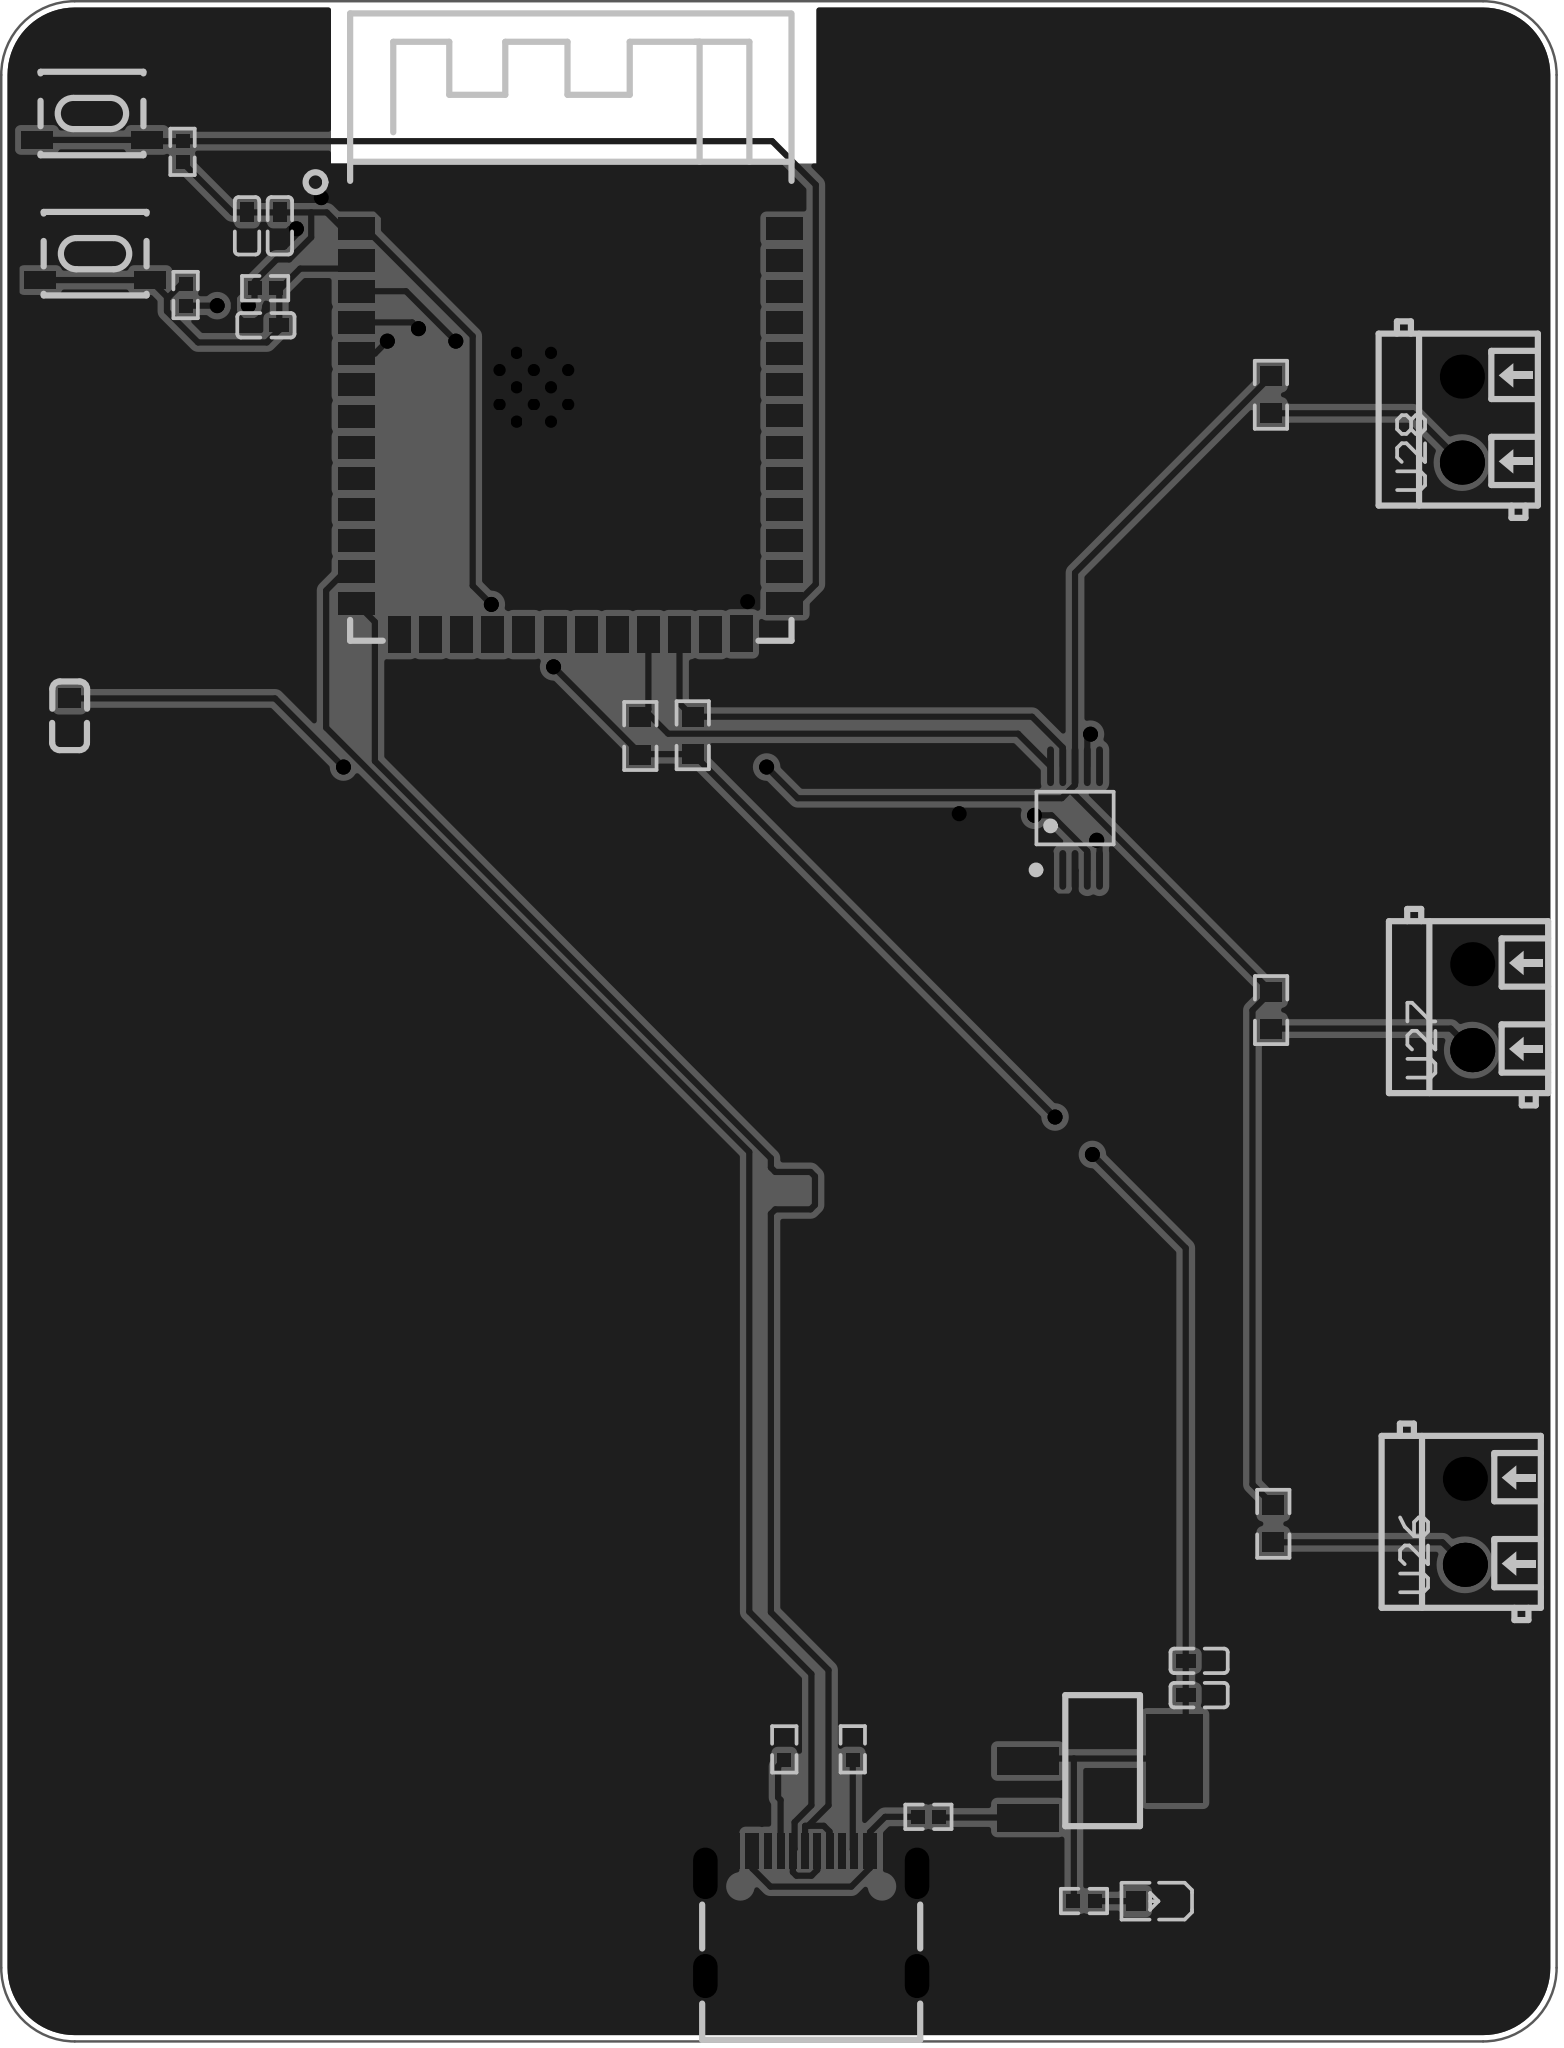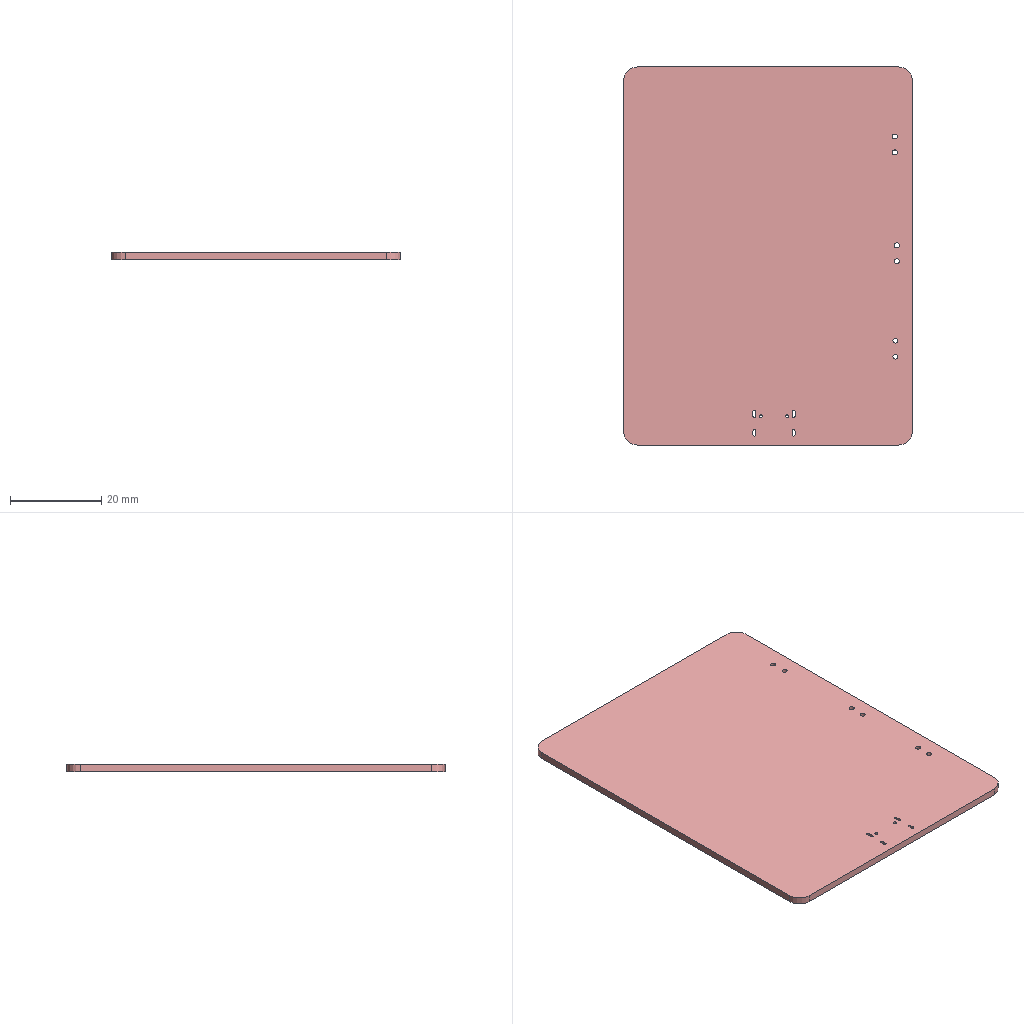Circuit board layout | Altium Designer | box 63.5 x 83.1 x 1.6 mm
Layer stack:
# Altium Designer layer stack of  (unit mm; dielectric type: 0 none, 1 core, 2 prepreg, 3 surface material)
index,name,kind,layer,copper_thickness_mm,dielectric_type,dielectric_thickness_mm,dielectric_material,dielectric_constant
0,Top Paste Mask Layer,other,,,,,,
1,Top Silkscreen Layer,other,,,,,,
2,Top Solder Mask Layer,dielectric,,,3,0.01,,3.3
3,Top Layer,copper,Top Layer,0.035,,,,
4,Dielectric1,dielectric,,,3,1.51,FR4,4.5
5,Bottom Layer,copper,Bottom Layer,0.035,,,,
6,Bottom Solder Mask Layer,dielectric,,,3,0.01,,3.3
7,Bottom Silkscreen Layer,other,,,,,,
8,Bottom Paste Mask Layer,other,,,,,,
# drill layer pairs: low layer,high layer
drill_pair,Top Layer,Bottom Layer
Part placement:
Designator,Comment,Layer,Footprint,Center-X(mm),Center-Y(mm),Rotation
C15,100nF,TopLayer,C0402,138.176,106.426,180
C16,10uF,TopLayer,C0402,138.176,105.029,180
C100,10uF,TopLayer,C0402,99.314,164.846,90
C101,100nF,TopLayer,C0402,100.654,164.847,90
C102,1uF,TopLayer,C0402,100.085,160.797,0
LED6,NCD0603R1,TopLayer,LED0603-RD_RED,136.398,96.647,180
R1,5.1K,TopLayer,r0402,121.245,102.821,90
R3,5.1K,TopLayer,r0402,124.039,102.824,90
R4,10K,TopLayer,r0402,133.477,96.647,0
R5,10K,TopLayer,r0402,96.68,167.859,90
R247,10K,TopLayer,r0402,96.807,162.029,90
R248,,TopLayer,r0402,100.053,162.306,180
R251,0,TopLayer,r0402,127.127,100.076,0
SW1,TS-1089S-02526,TopLayer,SW-SMD_4P-L4.2-W3.3-P2.15-LS5.1,92.986,169.419,0
SW3,TS-1089S-02526,TopLayer,SW-SMD_4P-L4.2-W3.3-P2.15-LS5.1,93.113,163.713,0
C30,100nF,TopLayer,C0603,92.075,144.907,90
U2,AMS1117-3.3,TopLayer,sot-223(gd32),134.191,102.348,270
U5,TYPE-C16P,TopLayer,USB-C-SMD_TYPE-C16PIN-SHOUHAN,122.342,96.144,0
U24,ESP32-S3-WROOM-1-N16R8,TopLayer,WIRELM-SMD_ESP32-S3-WROOM-1,112.522,157.099,0
R32,4.7K,TopLayer,R0603,117.507,144.108,270
R33,4.7K,TopLayer,R0603,115.369,144.077,270
R35,10K,TopLayer,R0603,141.206,112.005,90
R36,10K,TopLayer,R0603,141.116,132.919,90
R37,10K,TopLayer,R0603,141.108,157.968,90
U25,ADS1115IDGSR,TopLayer,MSOP-10_L3.0-W3.0-P0.50-LS5.0-BL,133.112,140.736,0
U26,DB301V-3.5-2P-GN-S,TopLayer,CONN-TH_DB301V-3.5-2P-GN,149.026,112.085,90
U27,DB301V-3.5-2P-GN-S,TopLayer,CONN-TH_DB301V-3.5-2P-GN,149.325,133.037,90
U28,DB301V-3.5-2P-GN-S,TopLayer,CONN-TH_DB301V-3.5-2P-GN,148.904,156.957,90
Pad and via stacks:
# Altium Designer via and pad stacks of  (unit mm). Each distinct definition once, with the count of objects using it.
# via: kind,start_layer,end_layer,hole_mm,diameter_mm,mode(0 simple;1 top-mid-bottom;2 full stack),diameter_per_layer,count,example_net
# pad: kind,layer,hole_mm,hole_type(0 round;1 square;2 slot),plating,top_size,top_shape(1 round;2 rect;3 octagon;9 rounded rect),mid_size,bottom_size,mode,footprint,size_per_layer,count,example
pad,Top Layer,0,0,plated,0.7901x0.54,2,0.7901x0.54,0.7901x0.54,0,C0402,,10,C15.2
pad,Top Layer,0,0,plated,0.8x0.8,2,0.8x0.8,0.8x0.8,0,LED0603-RD_RED,,2,LED6.1
pad,Top Layer,0,0,plated,0.5657x0.54,2,0.5657x0.54,0.5657x0.54,0,r0402,,14,R1.2
pad,Top Layer,0,0,plated,0.7x1.3,2,0.7x1.3,0.7x1.3,0,SW-SMD_4P-L4.2-W3.3-P2.15-LS5.1,,8,SW1.1
pad,Top Layer,0,0,plated,0.8x0.9,2,0.8x0.9,0.8x0.9,0,C0603,,2,C30.2
pad,Top Layer,0,0,plated,1.1x2.5,2,1.1x2.5,1.1x2.5,0,sot-223(gd32),,3,U2.1
pad,Top Layer,0,0,plated,3.6x2.29,2,3.6x2.29,3.6x2.29,0,sot-223(gd32),,1,U2.4
pad,Top Layer,0,0,plated,0.2997x1.45,2,0.2997x1.45,0.2997x1.45,0,USB-C-SMD_TYPE-C16PIN-SHOUHAN,,8,U5.B8
pad,Top Layer,0,0,plated,0.5512x1.45,2,0.5512x1.45,0.5512x1.45,0,USB-C-SMD_TYPE-C16PIN-SHOUHAN,,4,U5.B4A9
pad,Top Layer,0,0,plated,1.5x0.9,2,1.5x0.9,1.5x0.9,0,WIRELM-SMD_ESP32-S3-WROOM-1,,40,U24.1
pad,Top Layer,0,0,plated,0.9x0.9,2,0.9x0.9,0.9x0.9,0,WIRELM-SMD_ESP32-S3-WROOM-1,,9,U24.41
pad,Top Layer,0,0,plated,0.8065x0.864,2,0.8065x0.864,0.8065x0.864,0,R0603,,10,R32.2
pad,Top Layer,0,0,plated,0.28x1.62,1,0.28x1.62,0.28x1.62,0,MSOP-10_L3.0-W3.0-P0.50-LS5.0-BL,,10,U25.1
pad,Multi-Layer,0.5994,2,plated,1.001x1.801,1,1.001x1.801,1.001x1.801,0,USB-C-SMD_TYPE-C16PIN-SHOUHAN,,2,U5.4
pad,Multi-Layer,0.5994,2,plated,1.001x2.101,1,1.001x2.101,1.001x2.101,0,USB-C-SMD_TYPE-C16PIN-SHOUHAN,,2,U5.1
pad,Multi-Layer,1.1,0,plated,1.8x1.8,1,1.8x1.8,1.8x1.8,0,CONN-TH_DB301V-3.5-2P-GN,,6,U26.1
via,Top Layer,Bottom Layer,0.3048,0.61,0,,18,+3V3
via,Top Layer,Bottom Layer,0.2997,0.5,0,,12,GND
Copper pours:
name,layer,net,type(0 solid;1 hatched;2 none)
Bottom Layer-GND,Bottom Layer,GND,0
Top Layer-GND,Top Layer,GND,0
Design rules, without the lines most boards share:
# Altium Designer design rules of  (exported by Altium Designer, unit mm)
# columns: name | kind | enabled | priority | scope1 | scope2 | descriptor | typed fields (field=value)
copperRegion | 20 | enabled | 1 | All | All | Polygon Connect Rule(Direct Connect )(Conductor Width=10mil) (Relief Angle=90 Angle) (Entries=4) (Air Gap Width=10mil) (All),(All) | connect_style(0=relief,1=direct,2=none)=1 relief_conductor_width=0.254 relief_entries=4
solderMaskExpansion | 13 | enabled | 2 | All | All | Solder Mask Expansion (Expansion =2.008mil) (All) | expansion=0.051